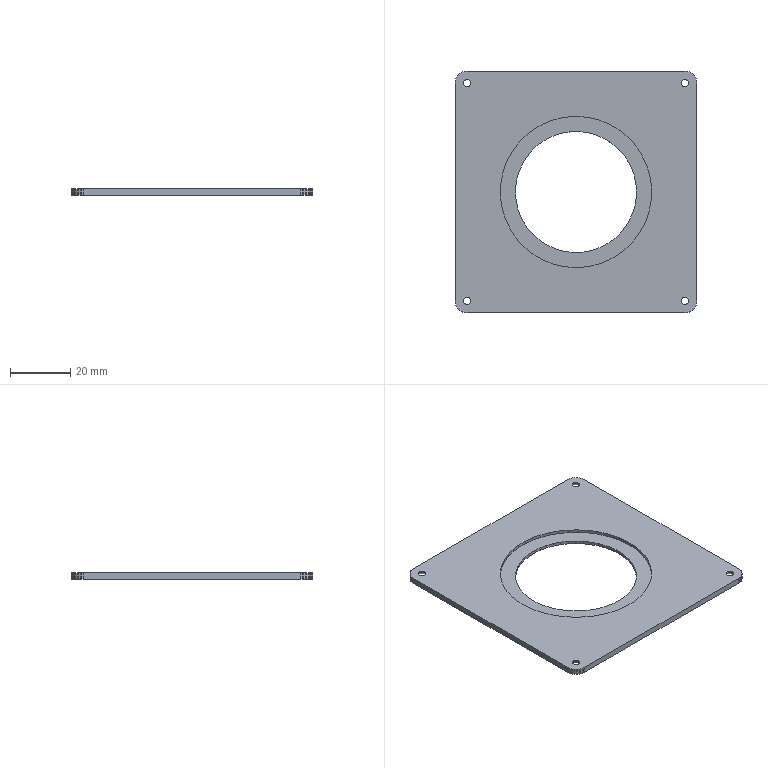Part | SolidWorks | features ICE 7, Chamfer 1, Extrusion 1, MoveFace 1 | 1 solid | 171 faces | box 80 x 80 x 2 mm | volume 9472 mm3 | plane 155 | cone 8 | cylinder 8 | commonest cylinder face diameters 2.5 x8